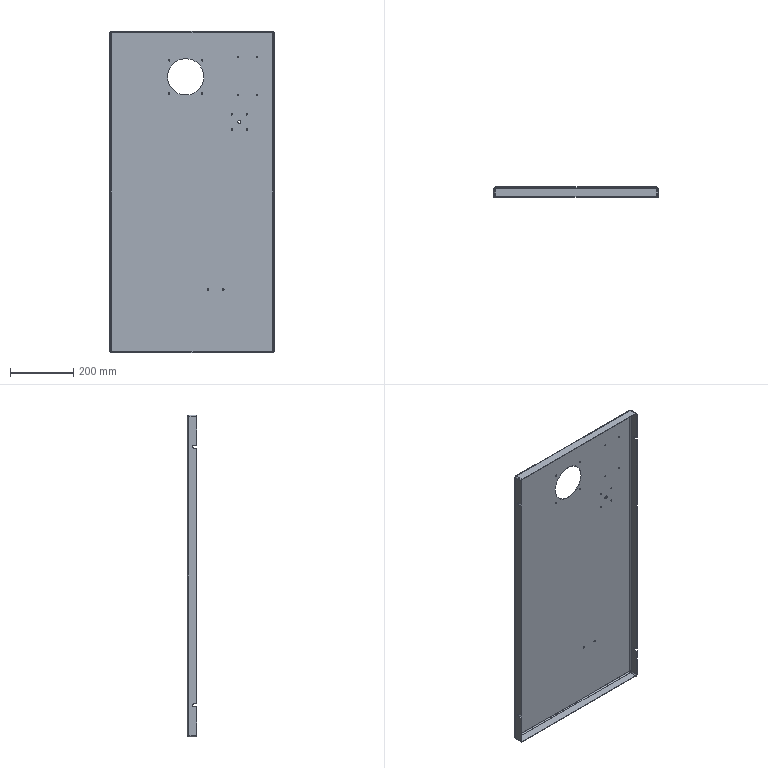Part | STEP file | 1 solid | 82 faces | box 520 x 30 x 1020 mm | volume 901440 mm3 | cylinder 52 | plane 22 | spline 8 | commonest cylinder face diameters 10 x10 3.6 x8 4.2 x8 4.5 x8 7 x8 5.5 x4